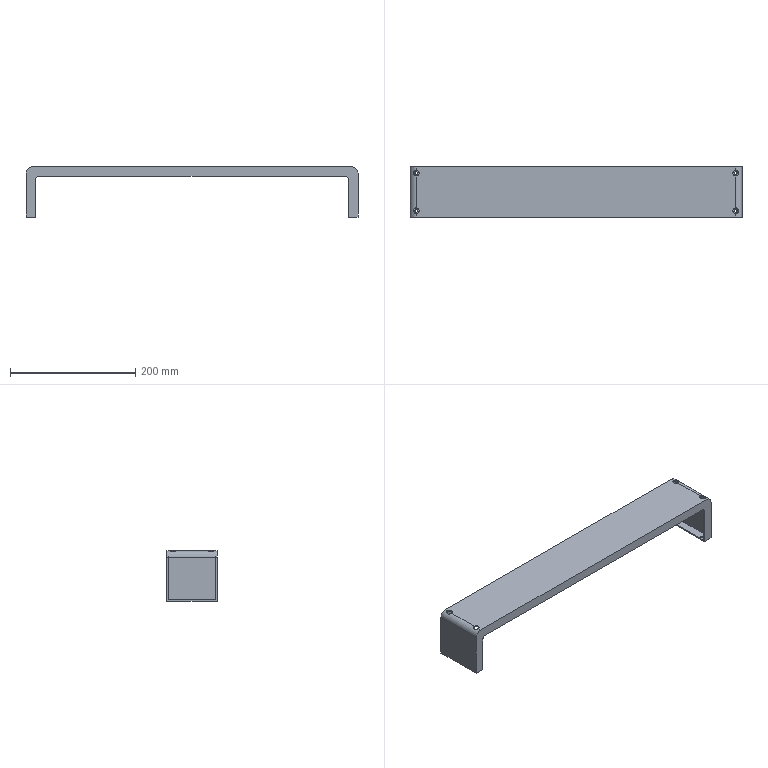Part | NX | 1 solid | 37 faces | box 530 x 80 x 80 mm | volume 145819 mm3 | cylinder 19 | plane 18 | commonest cylinder face diameters 4.5 x4 9 x4 10 x4 3.3 x3 16 x2 20 x2
STEP:
#1=CARTESIAN_POINT('',(-252.75,30.,-40.));
#2=VERTEX_POINT('',#1);
#3=CARTESIAN_POINT('',(-255.,30.,-40.));
#4=DIRECTION('',(0.,0.,1.));
#5=DIRECTION('',(1.,0.,0.));
#6=AXIS2_PLACEMENT_3D('',#3,#4,#5);
#7=CIRCLE('',#6,2.25);
#8=EDGE_CURVE('',#2,#2,#7,.T.);
#9=ORIENTED_EDGE('',*,*,#8,.T.);
#10=EDGE_LOOP('',(#9));
#11=FACE_BOUND('',#10,.T.);
#12=CARTESIAN_POINT('',(-252.75,-30.,-40.));
#13=VERTEX_POINT('',#12);
#14=CARTESIAN_POINT('',(-255.,-30.,-40.));
#15=DIRECTION('',(0.,0.,1.));
#16=DIRECTION('',(1.,0.,0.));
#17=AXIS2_PLACEMENT_3D('',#14,#15,#16);
#18=CIRCLE('',#17,2.25);
#19=EDGE_CURVE('',#13,#13,#18,.T.);
#20=ORIENTED_EDGE('',*,*,#19,.T.);
#21=EDGE_LOOP('',(#20));
#22=FACE_BOUND('',#21,.T.);
#23=CARTESIAN_POINT('',(-250.,40.,-40.));
#24=VERTEX_POINT('',#23);
#25=CARTESIAN_POINT('',(-265.,40.,-40.));
#26=VERTEX_POINT('',#25);
#27=CARTESIAN_POINT('',(-265.,40.,-40.));
#28=DIRECTION('',(-1.,0.,0.));
#29=VECTOR('',#28,1000.);
#30=LINE('',#27,#29);
#31=EDGE_CURVE('',#24,#26,#30,.T.);
#32=ORIENTED_EDGE('',*,*,#31,.F.);
#33=CARTESIAN_POINT('',(-250.,-40.,-40.));
#34=VERTEX_POINT('',#33);
#35=CARTESIAN_POINT('',(-250.,-40.,-40.));
#36=DIRECTION('',(0.,-1.,0.));
#37=VECTOR('',#36,1000.);
#38=LINE('',#35,#37);
#39=EDGE_CURVE('',#24,#34,#38,.T.);
#40=ORIENTED_EDGE('',*,*,#39,.T.);
#41=CARTESIAN_POINT('',(-265.,-40.,-40.));
#42=VERTEX_POINT('',#41);
#43=CARTESIAN_POINT('',(-265.,-40.,-40.));
#44=DIRECTION('',(-1.,0.,0.));
#45=VECTOR('',#44,1000.);
#46=LINE('',#43,#45);
#47=EDGE_CURVE('',#34,#42,#46,.T.);
#48=ORIENTED_EDGE('',*,*,#47,.T.);
#49=CARTESIAN_POINT('',(-265.,40.,-40.));
#50=DIRECTION('',(0.,-1.,0.));
#51=VECTOR('',#50,1000.);
#52=LINE('',#49,#51);
#53=EDGE_CURVE('',#26,#42,#52,.T.);
#54=ORIENTED_EDGE('',*,*,#53,.F.);
#55=EDGE_LOOP('',(#32,#40,#48,#54));
#56=FACE_BOUND('',#55,.T.);
#57=CARTESIAN_POINT('',(-265.,40.,-40.));
#58=DIRECTION('',(0.,0.,1.));
#59=DIRECTION('',(1.,0.,0.));
#60=AXIS2_PLACEMENT_3D('',#57,#58,#59);
#61=PLANE('',#60);
#62=ADVANCED_FACE('',(#11,#22,#56),#61,.F.);
#63=CARTESIAN_POINT('',(257.25,-30.,-40.));
#64=VERTEX_POINT('',#63);
#65=CARTESIAN_POINT('',(255.,-30.,-40.));
#66=DIRECTION('',(0.,0.,1.));
#67=DIRECTION('',(1.,0.,0.));
#68=AXIS2_PLACEMENT_3D('',#65,#66,#67);
#69=CIRCLE('',#68,2.25);
#70=EDGE_CURVE('',#64,#64,#69,.T.);
#71=ORIENTED_EDGE('',*,*,#70,.T.);
#72=EDGE_LOOP('',(#71));
#73=FACE_BOUND('',#72,.T.);
#74=CARTESIAN_POINT('',(257.25,30.,-40.));
#75=VERTEX_POINT('',#74);
#76=CARTESIAN_POINT('',(255.,30.,-40.));
#77=DIRECTION('',(0.,0.,1.));
#78=DIRECTION('',(1.,0.,0.));
#79=AXIS2_PLACEMENT_3D('',#76,#77,#78);
#80=CIRCLE('',#79,2.25);
#81=EDGE_CURVE('',#75,#75,#80,.T.);
#82=ORIENTED_EDGE('',*,*,#81,.T.);
#83=EDGE_LOOP('',(#82));
#84=FACE_BOUND('',#83,.T.);
#85=CARTESIAN_POINT('',(265.,-40.,-40.));
#86=VERTEX_POINT('',#85);
#87=CARTESIAN_POINT('',(250.,-40.,-40.));
#88=VERTEX_POINT('',#87);
#89=CARTESIAN_POINT('',(-265.,-40.,-40.));
#90=DIRECTION('',(-1.,0.,0.));
#91=VECTOR('',#90,1000.);
#92=LINE('',#89,#91);
#93=EDGE_CURVE('',#86,#88,#92,.T.);
#94=ORIENTED_EDGE('',*,*,#93,.T.);
#95=CARTESIAN_POINT('',(250.,40.,-40.));
#96=VERTEX_POINT('',#95);
#97=CARTESIAN_POINT('',(250.,-40.,-40.));
#98=DIRECTION('',(0.,1.,0.));
#99=VECTOR('',#98,1000.);
#100=LINE('',#97,#99);
#101=EDGE_CURVE('',#88,#96,#100,.T.);
#102=ORIENTED_EDGE('',*,*,#101,.T.);
#103=CARTESIAN_POINT('',(265.,40.,-40.));
#104=VERTEX_POINT('',#103);
#105=CARTESIAN_POINT('',(-265.,40.,-40.));
#106=DIRECTION('',(-1.,0.,0.));
#107=VECTOR('',#106,1000.);
#108=LINE('',#105,#107);
#109=EDGE_CURVE('',#104,#96,#108,.T.);
#110=ORIENTED_EDGE('',*,*,#109,.F.);
#111=CARTESIAN_POINT('',(265.,40.,-40.));
#112=DIRECTION('',(0.,-1.,0.));
#113=VECTOR('',#112,1000.);
#114=LINE('',#111,#113);
#115=EDGE_CURVE('',#104,#86,#114,.T.);
#116=ORIENTED_EDGE('',*,*,#115,.T.);
#117=EDGE_LOOP('',(#94,#102,#110,#116));
#118=FACE_BOUND('',#117,.T.);
#119=CARTESIAN_POINT('',(-265.,40.,-40.));
#120=DIRECTION('',(0.,0.,1.));
#121=DIRECTION('',(1.,0.,0.));
#122=AXIS2_PLACEMENT_3D('',#119,#120,#121);
#123=PLANE('',#122);
#124=ADVANCED_FACE('',(#73,#84,#118),#123,.F.);
#125=CARTESIAN_POINT('',(265.,-40.,30.));
#126=VERTEX_POINT('',#125);
#127=CARTESIAN_POINT('',(265.,-40.,-40.));
#128=DIRECTION('',(0.,0.,-1.));
#129=VECTOR('',#128,1000.);
#130=LINE('',#127,#129);
#131=EDGE_CURVE('',#126,#86,#130,.T.);
#132=ORIENTED_EDGE('',*,*,#131,.T.);
#133=ORIENTED_EDGE('',*,*,#115,.F.);
#134=CARTESIAN_POINT('',(265.,40.,30.));
#135=VERTEX_POINT('',#134);
#136=CARTESIAN_POINT('',(265.,40.,-40.));
#137=DIRECTION('',(0.,0.,-1.));
#138=VECTOR('',#137,1000.);
#139=LINE('',#136,#138);
#140=EDGE_CURVE('',#135,#104,#139,.T.);
#141=ORIENTED_EDGE('',*,*,#140,.F.);
#142=CARTESIAN_POINT('',(265.,40.,30.));
#143=DIRECTION('',(0.,-1.,0.));
#144=VECTOR('',#143,1000.);
#145=LINE('',#142,#144);
#146=EDGE_CURVE('',#135,#126,#145,.T.);
#147=ORIENTED_EDGE('',*,*,#146,.T.);
#148=EDGE_LOOP('',(#132,#133,#141,#147));
#149=FACE_BOUND('',#148,.T.);
#150=CARTESIAN_POINT('',(265.,40.,-40.));
#151=DIRECTION('',(-1.,0.,0.));
#152=DIRECTION('',(0.,0.,1.));
#153=AXIS2_PLACEMENT_3D('',#150,#151,#152);
#154=PLANE('',#153);
#155=ADVANCED_FACE('',(#149),#154,.F.);
#156=CARTESIAN_POINT('',(-265.,-40.,30.));
#157=VERTEX_POINT('',#156);
#158=CARTESIAN_POINT('',(-265.,40.,30.));
#159=VERTEX_POINT('',#158);
#160=CARTESIAN_POINT('',(-265.,40.,30.));
#161=DIRECTION('',(0.,-1.,0.));
#162=VECTOR('',#161,1000.);
#163=LINE('',#160,#162);
#164=EDGE_CURVE('',#157,#159,#163,.F.);
#165=ORIENTED_EDGE('',*,*,#164,.T.);
#166=CARTESIAN_POINT('',(-265.,40.,-40.));
#167=DIRECTION('',(0.,0.,1.));
#168=VECTOR('',#167,1000.);
#169=LINE('',#166,#168);
#170=EDGE_CURVE('',#26,#159,#169,.T.);
#171=ORIENTED_EDGE('',*,*,#170,.F.);
#172=ORIENTED_EDGE('',*,*,#53,.T.);
#173=CARTESIAN_POINT('',(-265.,-40.,-40.));
#174=DIRECTION('',(0.,0.,1.));
#175=VECTOR('',#174,1000.);
#176=LINE('',#173,#175);
#177=EDGE_CURVE('',#42,#157,#176,.T.);
#178=ORIENTED_EDGE('',*,*,#177,.T.);
#179=EDGE_LOOP('',(#165,#171,#172,#178));
#180=FACE_BOUND('',#179,.T.);
#181=CARTESIAN_POINT('',(-265.,40.,-40.));
#182=DIRECTION('',(1.,0.,0.));
#183=DIRECTION('',(0.,0.,-1.));
#184=AXIS2_PLACEMENT_3D('',#181,#182,#183);
#185=PLANE('',#184);
#186=ADVANCED_FACE('',(#180),#185,.F.);
#187=CARTESIAN_POINT('',(-255.,40.,40.));
#188=VERTEX_POINT('',#187);
#189=CARTESIAN_POINT('',(-255.,34.5,40.));
#190=VERTEX_POINT('',#189);
#191=CARTESIAN_POINT('',(-255.,40.,40.));
#192=DIRECTION('',(0.,-1.,0.));
#193=VECTOR('',#192,1000.);
#194=LINE('',#191,#193);
#195=EDGE_CURVE('',#188,#190,#194,.T.);
#196=ORIENTED_EDGE('',*,*,#195,.T.);
#197=CARTESIAN_POINT('',(-255.,25.5,40.));
#198=VERTEX_POINT('',#197);
#199=CARTESIAN_POINT('',(-255.,30.,40.));
#200=DIRECTION('',(0.,0.,1.));
#201=DIRECTION('',(1.,0.,0.));
#202=AXIS2_PLACEMENT_3D('',#199,#200,#201);
#203=CIRCLE('',#202,4.5);
#204=EDGE_CURVE('',#198,#190,#203,.T.);
#205=ORIENTED_EDGE('',*,*,#204,.F.);
#206=CARTESIAN_POINT('',(-255.,-25.5,40.));
#207=VERTEX_POINT('',#206);
#208=CARTESIAN_POINT('',(-255.,40.,40.));
#209=DIRECTION('',(0.,-1.,0.));
#210=VECTOR('',#209,1000.);
#211=LINE('',#208,#210);
#212=EDGE_CURVE('',#198,#207,#211,.T.);
#213=ORIENTED_EDGE('',*,*,#212,.T.);
#214=CARTESIAN_POINT('',(-255.,-34.5,40.));
#215=VERTEX_POINT('',#214);
#216=CARTESIAN_POINT('',(-255.,-30.,40.));
#217=DIRECTION('',(0.,0.,1.));
#218=DIRECTION('',(1.,0.,0.));
#219=AXIS2_PLACEMENT_3D('',#216,#217,#218);
#220=CIRCLE('',#219,4.5);
#221=EDGE_CURVE('',#215,#207,#220,.T.);
#222=ORIENTED_EDGE('',*,*,#221,.F.);
#223=CARTESIAN_POINT('',(-255.,-40.,40.));
#224=VERTEX_POINT('',#223);
#225=CARTESIAN_POINT('',(-255.,40.,40.));
#226=DIRECTION('',(0.,-1.,0.));
#227=VECTOR('',#226,1000.);
#228=LINE('',#225,#227);
#229=EDGE_CURVE('',#215,#224,#228,.T.);
#230=ORIENTED_EDGE('',*,*,#229,.T.);
#231=CARTESIAN_POINT('',(255.,-40.,40.));
#232=VERTEX_POINT('',#231);
#233=CARTESIAN_POINT('',(-265.,-40.,40.));
#234=DIRECTION('',(1.,0.,0.));
#235=VECTOR('',#234,1000.);
#236=LINE('',#233,#235);
#237=EDGE_CURVE('',#224,#232,#236,.T.);
#238=ORIENTED_EDGE('',*,*,#237,.T.);
#239=CARTESIAN_POINT('',(255.,-34.5,40.));
#240=VERTEX_POINT('',#239);
#241=CARTESIAN_POINT('',(255.,40.,40.));
#242=DIRECTION('',(0.,-1.,0.));
#243=VECTOR('',#242,1000.);
#244=LINE('',#241,#243);
#245=EDGE_CURVE('',#232,#240,#244,.F.);
#246=ORIENTED_EDGE('',*,*,#245,.T.);
#247=CARTESIAN_POINT('',(255.,-25.5,40.));
#248=VERTEX_POINT('',#247);
#249=CARTESIAN_POINT('',(255.,-30.,40.));
#250=DIRECTION('',(0.,0.,1.));
#251=DIRECTION('',(1.,0.,0.));
#252=AXIS2_PLACEMENT_3D('',#249,#250,#251);
#253=CIRCLE('',#252,4.5);
#254=EDGE_CURVE('',#248,#240,#253,.T.);
#255=ORIENTED_EDGE('',*,*,#254,.F.);
#256=CARTESIAN_POINT('',(255.,25.5,40.));
#257=VERTEX_POINT('',#256);
#258=CARTESIAN_POINT('',(255.,40.,40.));
#259=DIRECTION('',(0.,-1.,0.));
#260=VECTOR('',#259,1000.);
#261=LINE('',#258,#260);
#262=EDGE_CURVE('',#248,#257,#261,.F.);
#263=ORIENTED_EDGE('',*,*,#262,.T.);
#264=CARTESIAN_POINT('',(255.,34.5,40.));
#265=VERTEX_POINT('',#264);
#266=CARTESIAN_POINT('',(255.,30.,40.));
#267=DIRECTION('',(0.,0.,1.));
#268=DIRECTION('',(1.,0.,0.));
#269=AXIS2_PLACEMENT_3D('',#266,#267,#268);
#270=CIRCLE('',#269,4.5);
#271=EDGE_CURVE('',#265,#257,#270,.T.);
#272=ORIENTED_EDGE('',*,*,#271,.F.);
#273=CARTESIAN_POINT('',(255.,40.,40.));
#274=VERTEX_POINT('',#273);
#275=CARTESIAN_POINT('',(255.,40.,40.));
#276=DIRECTION('',(0.,-1.,0.));
#277=VECTOR('',#276,1000.);
#278=LINE('',#275,#277);
#279=EDGE_CURVE('',#265,#274,#278,.F.);
#280=ORIENTED_EDGE('',*,*,#279,.T.);
#281=CARTESIAN_POINT('',(-265.,40.,40.));
#282=DIRECTION('',(1.,0.,0.));
#283=VECTOR('',#282,1000.);
#284=LINE('',#281,#283);
#285=EDGE_CURVE('',#188,#274,#284,.T.);
#286=ORIENTED_EDGE('',*,*,#285,.F.);
#287=EDGE_LOOP('',(#196,#205,#213,#222,#230,#238,#246,#255,#263,#272,#280,#286));
#288=FACE_BOUND('',#287,.T.);
#289=CARTESIAN_POINT('',(-265.,40.,40.));
#290=DIRECTION('',(0.,0.,-1.));
#291=DIRECTION('',(-1.,0.,0.));
#292=AXIS2_PLACEMENT_3D('',#289,#290,#291);
#293=PLANE('',#292);
#294=ADVANCED_FACE('',(#288),#293,.F.);
#295=CARTESIAN_POINT('',(-255.,40.,31.65));
#296=VERTEX_POINT('',#295);
#297=CARTESIAN_POINT('',(-255.,40.,30.));
#298=DIRECTION('',(0.,1.,0.));
#299=DIRECTION('',(0.,0.,1.));
#300=AXIS2_PLACEMENT_3D('',#297,#298,#299);
#301=CIRCLE('',#300,1.65);
#302=EDGE_CURVE('',#296,#296,#301,.T.);
#303=ORIENTED_EDGE('',*,*,#302,.F.);
#304=EDGE_LOOP('',(#303));
#305=FACE_BOUND('',#304,.T.);
#306=CARTESIAN_POINT('',(0.,40.,31.65));
#307=VERTEX_POINT('',#306);
#308=CARTESIAN_POINT('',(0.,40.,30.));
#309=DIRECTION('',(0.,1.,0.));
#310=DIRECTION('',(0.,0.,1.));
#311=AXIS2_PLACEMENT_3D('',#308,#309,#310);
#312=CIRCLE('',#311,1.65);
#313=EDGE_CURVE('',#307,#307,#312,.T.);
#314=ORIENTED_EDGE('',*,*,#313,.F.);
#315=EDGE_LOOP('',(#314));
#316=FACE_BOUND('',#315,.T.);
#317=CARTESIAN_POINT('',(255.,40.,31.65));
#318=VERTEX_POINT('',#317);
#319=CARTESIAN_POINT('',(255.,40.,30.));
#320=DIRECTION('',(0.,1.,0.));
#321=DIRECTION('',(0.,0.,1.));
#322=AXIS2_PLACEMENT_3D('',#319,#320,#321);
#323=CIRCLE('',#322,1.65);
#324=EDGE_CURVE('',#318,#318,#323,.T.);
#325=ORIENTED_EDGE('',*,*,#324,.F.);
#326=EDGE_LOOP('',(#325));
#327=FACE_BOUND('',#326,.T.);
#328=CARTESIAN_POINT('',(-250.,40.,20.));
#329=VERTEX_POINT('',#328);
#330=CARTESIAN_POINT('',(-250.,40.,-40.));
#331=DIRECTION('',(0.,0.,1.));
#332=VECTOR('',#331,1000.);
#333=LINE('',#330,#332);
#334=EDGE_CURVE('',#24,#329,#333,.T.);
#335=ORIENTED_EDGE('',*,*,#334,.F.);
#336=ORIENTED_EDGE('',*,*,#31,.T.);
#337=ORIENTED_EDGE('',*,*,#170,.T.);
#338=CARTESIAN_POINT('',(-255.,40.,30.));
#339=DIRECTION('',(0.,1.,0.));
#340=DIRECTION('',(0.,0.,1.));
#341=AXIS2_PLACEMENT_3D('',#338,#339,#340);
#342=CIRCLE('',#341,10.);
#343=EDGE_CURVE('',#159,#188,#342,.T.);
#344=ORIENTED_EDGE('',*,*,#343,.T.);
#345=ORIENTED_EDGE('',*,*,#285,.T.);
#346=CARTESIAN_POINT('',(255.,40.,30.));
#347=DIRECTION('',(0.,1.,0.));
#348=DIRECTION('',(0.,0.,1.));
#349=AXIS2_PLACEMENT_3D('',#346,#347,#348);
#350=CIRCLE('',#349,10.);
#351=EDGE_CURVE('',#274,#135,#350,.T.);
#352=ORIENTED_EDGE('',*,*,#351,.T.);
#353=ORIENTED_EDGE('',*,*,#140,.T.);
#354=ORIENTED_EDGE('',*,*,#109,.T.);
#355=CARTESIAN_POINT('',(250.,40.,20.));
#356=VERTEX_POINT('',#355);
#357=CARTESIAN_POINT('',(250.,40.,-40.));
#358=DIRECTION('',(0.,0.,-1.));
#359=VECTOR('',#358,1000.);
#360=LINE('',#357,#359);
#361=EDGE_CURVE('',#356,#96,#360,.T.);
#362=ORIENTED_EDGE('',*,*,#361,.F.);
#363=CARTESIAN_POINT('',(245.,40.,25.));
#364=VERTEX_POINT('',#363);
#365=CARTESIAN_POINT('',(245.,40.,20.));
#366=DIRECTION('',(0.,1.,0.));
#367=DIRECTION('',(0.,0.,-1.));
#368=AXIS2_PLACEMENT_3D('',#365,#366,#367);
#369=CIRCLE('',#368,5.);
#370=EDGE_CURVE('',#364,#356,#369,.T.);
#371=ORIENTED_EDGE('',*,*,#370,.F.);
#372=CARTESIAN_POINT('',(-245.,40.,25.));
#373=VERTEX_POINT('',#372);
#374=CARTESIAN_POINT('',(-245.,40.,25.));
#375=DIRECTION('',(1.,0.,0.));
#376=VECTOR('',#375,1000.);
#377=LINE('',#374,#376);
#378=EDGE_CURVE('',#373,#364,#377,.T.);
#379=ORIENTED_EDGE('',*,*,#378,.F.);
#380=CARTESIAN_POINT('',(-245.,40.,20.));
#381=DIRECTION('',(0.,1.,0.));
#382=DIRECTION('',(0.,0.,-1.));
#383=AXIS2_PLACEMENT_3D('',#380,#381,#382);
#384=CIRCLE('',#383,5.);
#385=EDGE_CURVE('',#329,#373,#384,.T.);
#386=ORIENTED_EDGE('',*,*,#385,.F.);
#387=EDGE_LOOP('',(#335,#336,#337,#344,#345,#352,#353,#354,#362,#371,#379,#386));
#388=FACE_BOUND('',#387,.T.);
#389=CARTESIAN_POINT('',(0.,40.,0.));
#390=DIRECTION('',(0.,1.,0.));
#391=DIRECTION('',(0.,0.,1.));
#392=AXIS2_PLACEMENT_3D('',#389,#390,#391);
#393=PLANE('',#392);
#394=ADVANCED_FACE('',(#305,#316,#327,#388),#393,.T.);
#395=ORIENTED_EDGE('',*,*,#47,.F.);
#396=CARTESIAN_POINT('',(-250.,-40.,20.));
#397=VERTEX_POINT('',#396);
#398=CARTESIAN_POINT('',(-250.,-40.,-40.));
#399=DIRECTION('',(0.,0.,1.));
#400=VECTOR('',#399,1000.);
#401=LINE('',#398,#400);
#402=EDGE_CURVE('',#34,#397,#401,.T.);
#403=ORIENTED_EDGE('',*,*,#402,.T.);
#404=CARTESIAN_POINT('',(-245.,-40.,25.));
#405=VERTEX_POINT('',#404);
#406=CARTESIAN_POINT('',(-245.,-40.,20.));
#407=DIRECTION('',(0.,1.,0.));
#408=DIRECTION('',(0.,0.,-1.));
#409=AXIS2_PLACEMENT_3D('',#406,#407,#408);
#410=CIRCLE('',#409,5.);
#411=EDGE_CURVE('',#397,#405,#410,.T.);
#412=ORIENTED_EDGE('',*,*,#411,.T.);
#413=CARTESIAN_POINT('',(245.,-40.,25.));
#414=VERTEX_POINT('',#413);
#415=CARTESIAN_POINT('',(-245.,-40.,25.));
#416=DIRECTION('',(1.,0.,0.));
#417=VECTOR('',#416,1000.);
#418=LINE('',#415,#417);
#419=EDGE_CURVE('',#405,#414,#418,.T.);
#420=ORIENTED_EDGE('',*,*,#419,.T.);
#421=CARTESIAN_POINT('',(250.,-40.,20.));
#422=VERTEX_POINT('',#421);
#423=CARTESIAN_POINT('',(245.,-40.,20.));
#424=DIRECTION('',(0.,1.,0.));
#425=DIRECTION('',(0.,0.,-1.));
#426=AXIS2_PLACEMENT_3D('',#423,#424,#425);
#427=CIRCLE('',#426,5.);
#428=EDGE_CURVE('',#414,#422,#427,.T.);
#429=ORIENTED_EDGE('',*,*,#428,.T.);
#430=CARTESIAN_POINT('',(250.,-40.,-40.));
#431=DIRECTION('',(0.,0.,-1.));
#432=VECTOR('',#431,1000.);
#433=LINE('',#430,#432);
#434=EDGE_CURVE('',#422,#88,#433,.T.);
#435=ORIENTED_EDGE('',*,*,#434,.T.);
#436=ORIENTED_EDGE('',*,*,#93,.F.);
#437=ORIENTED_EDGE('',*,*,#131,.F.);
#438=CARTESIAN_POINT('',(255.,-40.,30.));
#439=DIRECTION('',(0.,1.,0.));
#440=DIRECTION('',(0.,0.,1.));
#441=AXIS2_PLACEMENT_3D('',#438,#439,#440);
#442=CIRCLE('',#441,10.);
#443=EDGE_CURVE('',#126,#232,#442,.F.);
#444=ORIENTED_EDGE('',*,*,#443,.T.);
#445=ORIENTED_EDGE('',*,*,#237,.F.);
#446=CARTESIAN_POINT('',(-255.,-40.,30.));
#447=DIRECTION('',(0.,1.,0.));
#448=DIRECTION('',(0.,0.,1.));
#449=AXIS2_PLACEMENT_3D('',#446,#447,#448);
#450=CIRCLE('',#449,10.);
#451=EDGE_CURVE('',#224,#157,#450,.F.);
#452=ORIENTED_EDGE('',*,*,#451,.T.);
#453=ORIENTED_EDGE('',*,*,#177,.F.);
#454=EDGE_LOOP('',(#395,#403,#412,#420,#429,#435,#436,#437,#444,#445,#452,#453));
#455=FACE_BOUND('',#454,.T.);
#456=CARTESIAN_POINT('',(0.,-40.,0.));
#457=DIRECTION('',(0.,1.,0.));
#458=DIRECTION('',(0.,0.,1.));
#459=AXIS2_PLACEMENT_3D('',#456,#457,#458);
#460=PLANE('',#459);
#461=ADVANCED_FACE('',(#455),#460,.F.);
#462=CARTESIAN_POINT('',(-255.,34.5,40.));
#463=CARTESIAN_POINT('',(-256.206,34.5,40.));
#464=CARTESIAN_POINT('',(-258.514,33.52,39.494));
#465=CARTESIAN_POINT('',(-259.992,30.011,38.648));
#466=CARTESIAN_POINT('',(-258.516,26.475,39.493));
#467=CARTESIAN_POINT('',(-256.207,25.5,40.));
#468=CARTESIAN_POINT('',(-255.,25.5,40.));
#469=B_SPLINE_CURVE_WITH_KNOTS('',3,(#462,#463,#464,#465,#466,#467,#468),.UNSPECIFIED.,.F.,.F.,(4,1,1,1,4),(0.,0.003564,0.007128,0.01069,0.01426),.UNSPECIFIED.);
#470=EDGE_CURVE('',#190,#198,#469,.T.);
#471=ORIENTED_EDGE('',*,*,#470,.F.);
#472=ORIENTED_EDGE('',*,*,#195,.F.);
#473=ORIENTED_EDGE('',*,*,#343,.F.);
#474=ORIENTED_EDGE('',*,*,#164,.F.);
#475=ORIENTED_EDGE('',*,*,#451,.F.);
#476=ORIENTED_EDGE('',*,*,#229,.F.);
#477=CARTESIAN_POINT('',(-255.,-25.5,40.));
#478=CARTESIAN_POINT('',(-256.206,-25.5,40.));
#479=CARTESIAN_POINT('',(-258.514,-26.48,39.494));
#480=CARTESIAN_POINT('',(-259.992,-29.989,38.648));
#481=CARTESIAN_POINT('',(-258.516,-33.525,39.493));
#482=CARTESIAN_POINT('',(-256.207,-34.5,40.));
#483=CARTESIAN_POINT('',(-255.,-34.5,40.));
#484=B_SPLINE_CURVE_WITH_KNOTS('',3,(#477,#478,#479,#480,#481,#482,#483),.UNSPECIFIED.,.F.,.F.,(4,1,1,1,4),(0.,0.003564,0.007128,0.01069,0.01426),.UNSPECIFIED.);
#485=EDGE_CURVE('',#207,#215,#484,.T.);
#486=ORIENTED_EDGE('',*,*,#485,.F.);
#487=ORIENTED_EDGE('',*,*,#212,.F.);
#488=EDGE_LOOP('',(#471,#472,#473,#474,#475,#476,#486,#487));
#489=FACE_BOUND('',#488,.T.);
#490=CARTESIAN_POINT('',(-255.,40.,30.));
#491=DIRECTION('',(0.,-1.,0.));
#492=DIRECTION('',(0.,0.,-1.));
#493=AXIS2_PLACEMENT_3D('',#490,#491,#492);
#494=CYLINDRICAL_SURFACE('',#493,10.);
#495=ADVANCED_FACE('',(#489),#494,.T.);
#496=CARTESIAN_POINT('',(255.,-34.5,40.));
#497=CARTESIAN_POINT('',(256.206,-34.5,40.));
#498=CARTESIAN_POINT('',(258.514,-33.52,39.494));
#499=CARTESIAN_POINT('',(259.992,-30.011,38.648));
#500=CARTESIAN_POINT('',(258.516,-26.475,39.493));
#501=CARTESIAN_POINT('',(256.207,-25.5,40.));
#502=CARTESIAN_POINT('',(255.,-25.5,40.));
#503=B_SPLINE_CURVE_WITH_KNOTS('',3,(#496,#497,#498,#499,#500,#501,#502),.UNSPECIFIED.,.F.,.F.,(4,1,1,1,4),(0.,0.003564,0.007128,0.01069,0.01426),.UNSPECIFIED.);
#504=EDGE_CURVE('',#240,#248,#503,.T.);
#505=ORIENTED_EDGE('',*,*,#504,.F.);
#506=ORIENTED_EDGE('',*,*,#245,.F.);
#507=ORIENTED_EDGE('',*,*,#443,.F.);
#508=ORIENTED_EDGE('',*,*,#146,.F.);
#509=ORIENTED_EDGE('',*,*,#351,.F.);
#510=ORIENTED_EDGE('',*,*,#279,.F.);
#511=CARTESIAN_POINT('',(255.,25.5,40.));
#512=CARTESIAN_POINT('',(256.206,25.5,40.));
#513=CARTESIAN_POINT('',(258.514,26.48,39.494));
#514=CARTESIAN_POINT('',(259.992,29.989,38.648));
#515=CARTESIAN_POINT('',(258.516,33.525,39.493));
#516=CARTESIAN_POINT('',(256.207,34.5,40.));
#517=CARTESIAN_POINT('',(255.,34.5,40.));
#518=B_SPLINE_CURVE_WITH_KNOTS('',3,(#511,#512,#513,#514,#515,#516,#517),.UNSPECIFIED.,.F.,.F.,(4,1,1,1,4),(0.,0.003564,0.007128,0.01069,0.01426),.UNSPECIFIED.);
#519=EDGE_CURVE('',#257,#265,#518,.T.);
#520=ORIENTED_EDGE('',*,*,#519,.F.);
#521=ORIENTED_EDGE('',*,*,#262,.F.);
#522=EDGE_LOOP('',(#505,#506,#507,#508,#509,#510,#520,#521));
#523=FACE_BOUND('',#522,.T.);
#524=CARTESIAN_POINT('',(255.,40.,30.));
#525=DIRECTION('',(0.,-1.,0.));
#526=DIRECTION('',(0.,0.,-1.));
#527=AXIS2_PLACEMENT_3D('',#524,#525,#526);
#528=CYLINDRICAL_SURFACE('',#527,10.);
#529=ADVANCED_FACE('',(#523),#528,.T.);
#530=CARTESIAN_POINT('',(263.,-38.,-38.));
#531=VERTEX_POINT('',#530);
#532=CARTESIAN_POINT('',(263.,38.,-38.));
#533=VERTEX_POINT('',#532);
#534=CARTESIAN_POINT('',(263.,40.,-38.));
#535=DIRECTION('',(0.,1.,0.));
#536=VECTOR('',#535,1000.);
#537=LINE('',#534,#536);
#538=EDGE_CURVE('',#531,#533,#537,.T.);
#539=ORIENTED_EDGE('',*,*,#538,.F.);
#540=CARTESIAN_POINT('',(263.,-38.,30.));
#541=VERTEX_POINT('',#540);
#542=CARTESIAN_POINT('',(263.,-38.,-40.));
#543=DIRECTION('',(0.,0.,-1.));
#544=VECTOR('',#543,1000.);
#545=LINE('',#542,#544);
#546=EDGE_CURVE('',#541,#531,#545,.T.);
#547=ORIENTED_EDGE('',*,*,#546,.F.);
#548=CARTESIAN_POINT('',(263.,38.,30.));
#549=VERTEX_POINT('',#548);
#550=CARTESIAN_POINT('',(263.,40.,30.));
#551=DIRECTION('',(0.,1.,0.));
#552=VECTOR('',#551,1000.);
#553=LINE('',#550,#552);
#554=EDGE_CURVE('',#549,#541,#553,.F.);
#555=ORIENTED_EDGE('',*,*,#554,.F.);
#556=CARTESIAN_POINT('',(263.,38.,-40.));
#557=DIRECTION('',(0.,0.,-1.));
#558=VECTOR('',#557,1000.);
#559=LINE('',#556,#558);
#560=EDGE_CURVE('',#549,#533,#559,.T.);
#561=ORIENTED_EDGE('',*,*,#560,.T.);
#562=EDGE_LOOP('',(#539,#547,#555,#561));
#563=FACE_BOUND('',#562,.T.);
#564=CARTESIAN_POINT('',(263.,40.,-40.));
#565=DIRECTION('',(-1.,0.,0.));
#566=DIRECTION('',(0.,0.,1.));
#567=AXIS2_PLACEMENT_3D('',#564,#565,#566);
#568=PLANE('',#567);
#569=ADVANCED_FACE('',(#563),#568,.T.);
#570=CARTESIAN_POINT('',(-263.,38.,-38.));
#571=VERTEX_POINT('',#570);
#572=CARTESIAN_POINT('',(-263.,-38.,-38.));
#573=VERTEX_POINT('',#572);
#574=CARTESIAN_POINT('',(-263.,40.,-38.));
#575=DIRECTION('',(0.,-1.,0.));
#576=VECTOR('',#575,1000.);
#577=LINE('',#574,#576);
#578=EDGE_CURVE('',#571,#573,#577,.T.);
#579=ORIENTED_EDGE('',*,*,#578,.F.);
#580=CARTESIAN_POINT('',(-263.,38.,30.));
#581=VERTEX_POINT('',#580);
#582=CARTESIAN_POINT('',(-263.,38.,-40.));
#583=DIRECTION('',(0.,0.,1.));
#584=VECTOR('',#583,1000.);
#585=LINE('',#582,#584);
#586=EDGE_CURVE('',#571,#581,#585,.T.);
#587=ORIENTED_EDGE('',*,*,#586,.T.);
#588=CARTESIAN_POINT('',(-263.,-38.,30.));
#589=VERTEX_POINT('',#588);
#590=CARTESIAN_POINT('',(-263.,40.,30.));
#591=DIRECTION('',(0.,1.,0.));
#592=VECTOR('',#591,1000.);
#593=LINE('',#590,#592);
#594=EDGE_CURVE('',#589,#581,#593,.T.);
#595=ORIENTED_EDGE('',*,*,#594,.F.);
#596=CARTESIAN_POINT('',(-263.,-38.,-40.));
#597=DIRECTION('',(0.,0.,1.));
#598=VECTOR('',#597,1000.);
#599=LINE('',#596,#598);
#600=EDGE_CURVE('',#573,#589,#599,.T.);
#601=ORIENTED_EDGE('',*,*,#600,.F.);
#602=EDGE_LOOP('',(#579,#587,#595,#601));
#603=FACE_BOUND('',#602,.T.);
#604=CARTESIAN_POINT('',(-263.,40.,-40.));
#605=DIRECTION('',(1.,0.,0.));
#606=DIRECTION('',(0.,0.,-1.));
#607=AXIS2_PLACEMENT_3D('',#604,#605,#606);
#608=PLANE('',#607);
#609=ADVANCED_FACE('',(#603),#608,.T.);
#610=CARTESIAN_POINT('',(-255.,34.5,38.));
#611=VERTEX_POINT('',#610);
#612=CARTESIAN_POINT('',(-255.,25.5,38.));
#613=VERTEX_POINT('',#612);
#614=CARTESIAN_POINT('',(-255.,30.,38.));
#615=DIRECTION('',(0.,0.,-1.));
#616=DIRECTION('',(-1.,0.,0.));
#617=AXIS2_PLACEMENT_3D('',#614,#615,#616);
#618=CIRCLE('',#617,4.5);
#619=EDGE_CURVE('',#611,#613,#618,.T.);
#620=ORIENTED_EDGE('',*,*,#619,.F.);
#621=CARTESIAN_POINT('',(-255.,38.,38.));
#622=VERTEX_POINT('',#621);
#623=CARTESIAN_POINT('',(-255.,40.,38.));
#624=DIRECTION('',(0.,1.,0.));
#625=VECTOR('',#624,1000.);
#626=LINE('',#623,#625);
#627=EDGE_CURVE('',#622,#611,#626,.F.);
#628=ORIENTED_EDGE('',*,*,#627,.F.);
#629=CARTESIAN_POINT('',(255.,38.,38.));
#630=VERTEX_POINT('',#629);
#631=CARTESIAN_POINT('',(-265.,38.,38.));
#632=DIRECTION('',(1.,0.,0.));
#633=VECTOR('',#632,1000.);
#634=LINE('',#631,#633);
#635=EDGE_CURVE('',#622,#630,#634,.T.);
#636=ORIENTED_EDGE('',*,*,#635,.T.);
#637=CARTESIAN_POINT('',(255.,34.5,38.));
#638=VERTEX_POINT('',#637);
#639=CARTESIAN_POINT('',(255.,40.,38.));
#640=DIRECTION('',(0.,1.,0.));
#641=VECTOR('',#640,1000.);
#642=LINE('',#639,#641);
#643=EDGE_CURVE('',#638,#630,#642,.T.);
#644=ORIENTED_EDGE('',*,*,#643,.F.);
#645=CARTESIAN_POINT('',(255.,25.5,38.));
#646=VERTEX_POINT('',#645);
#647=CARTESIAN_POINT('',(255.,30.,38.));
#648=DIRECTION('',(0.,0.,-1.));
#649=DIRECTION('',(-1.,0.,0.));
#650=AXIS2_PLACEMENT_3D('',#647,#648,#649);
#651=CIRCLE('',#650,4.5);
#652=EDGE_CURVE('',#646,#638,#651,.T.);
#653=ORIENTED_EDGE('',*,*,#652,.F.);
#654=CARTESIAN_POINT('',(255.,-25.5,38.));
#655=VERTEX_POINT('',#654);
#656=CARTESIAN_POINT('',(255.,40.,38.));
#657=DIRECTION('',(0.,1.,0.));
#658=VECTOR('',#657,1000.);
#659=LINE('',#656,#658);
#660=EDGE_CURVE('',#655,#646,#659,.T.);
#661=ORIENTED_EDGE('',*,*,#660,.F.);
#662=CARTESIAN_POINT('',(255.,-34.5,38.));
#663=VERTEX_POINT('',#662);
#664=CARTESIAN_POINT('',(255.,-30.,38.));
#665=DIRECTION('',(0.,0.,-1.));
#666=DIRECTION('',(-1.,0.,0.));
#667=AXIS2_PLACEMENT_3D('',#664,#665,#666);
#668=CIRCLE('',#667,4.5);
#669=EDGE_CURVE('',#663,#655,#668,.T.);
#670=ORIENTED_EDGE('',*,*,#669,.F.);
#671=CARTESIAN_POINT('',(255.,-38.,38.));
#672=VERTEX_POINT('',#671);
#673=CARTESIAN_POINT('',(255.,40.,38.));
#674=DIRECTION('',(0.,1.,0.));
#675=VECTOR('',#674,1000.);
#676=LINE('',#673,#675);
#677=EDGE_CURVE('',#672,#663,#676,.T.);
#678=ORIENTED_EDGE('',*,*,#677,.F.);
#679=CARTESIAN_POINT('',(-255.,-38.,38.));
#680=VERTEX_POINT('',#679);
#681=CARTESIAN_POINT('',(-265.,-38.,38.));
#682=DIRECTION('',(1.,0.,0.));
#683=VECTOR('',#682,1000.);
#684=LINE('',#681,#683);
#685=EDGE_CURVE('',#680,#672,#684,.T.);
#686=ORIENTED_EDGE('',*,*,#685,.F.);
#687=CARTESIAN_POINT('',(-255.,-34.5,38.));
#688=VERTEX_POINT('',#687);
#689=CARTESIAN_POINT('',(-255.,40.,38.));
#690=DIRECTION('',(0.,1.,0.));
#691=VECTOR('',#690,1000.);
#692=LINE('',#689,#691);
#693=EDGE_CURVE('',#688,#680,#692,.F.);
#694=ORIENTED_EDGE('',*,*,#693,.F.);
#695=CARTESIAN_POINT('',(-255.,-25.5,38.));
#696=VERTEX_POINT('',#695);
#697=CARTESIAN_POINT('',(-255.,-30.,38.));
#698=DIRECTION('',(0.,0.,-1.));
#699=DIRECTION('',(-1.,0.,0.));
#700=AXIS2_PLACEMENT_3D('',#697,#698,#699);
#701=CIRCLE('',#700,4.5);
#702=EDGE_CURVE('',#696,#688,#701,.T.);
#703=ORIENTED_EDGE('',*,*,#702,.F.);
#704=CARTESIAN_POINT('',(-255.,40.,38.));
#705=DIRECTION('',(0.,1.,0.));
#706=VECTOR('',#705,1000.);
#707=LINE('',#704,#706);
#708=EDGE_CURVE('',#613,#696,#707,.F.);
#709=ORIENTED_EDGE('',*,*,#708,.F.);
#710=EDGE_LOOP('',(#620,#628,#636,#644,#653,#661,#670,#678,#686,#694,#703,#709));
#711=FACE_BOUND('',#710,.T.);
#712=CARTESIAN_POINT('',(-265.,40.,38.));
#713=DIRECTION('',(0.,0.,-1.));
#714=DIRECTION('',(-1.,0.,0.));
#715=AXIS2_PLACEMENT_3D('',#712,#713,#714);
#716=PLANE('',#715);
#717=ADVANCED_FACE('',(#711),#716,.T.);
#718=CARTESIAN_POINT('',(-255.,38.,31.65));
#719=VERTEX_POINT('',#718);
#720=CARTESIAN_POINT('',(-255.,38.,30.));
#721=DIRECTION('',(0.,1.,0.));
#722=DIRECTION('',(0.,0.,1.));
#723=AXIS2_PLACEMENT_3D('',#720,#721,#722);
#724=CIRCLE('',#723,1.65);
#725=EDGE_CURVE('',#719,#719,#724,.T.);
#726=ORIENTED_EDGE('',*,*,#725,.T.);
#727=EDGE_LOOP('',(#726));
#728=FACE_BOUND('',#727,.T.);
#729=CARTESIAN_POINT('',(0.,38.,31.65));
#730=VERTEX_POINT('',#729);
#731=CARTESIAN_POINT('',(0.,38.,30.));
#732=DIRECTION('',(0.,1.,0.));
#733=DIRECTION('',(0.,0.,1.));
#734=AXIS2_PLACEMENT_3D('',#731,#732,#733);
#735=CIRCLE('',#734,1.65);
#736=EDGE_CURVE('',#730,#730,#735,.T.);
#737=ORIENTED_EDGE('',*,*,#736,.T.);
#738=EDGE_LOOP('',(#737));
#739=FACE_BOUND('',#738,.T.);
#740=CARTESIAN_POINT('',(255.,38.,31.65));
#741=VERTEX_POINT('',#740);
#742=CARTESIAN_POINT('',(255.,38.,30.));
#743=DIRECTION('',(0.,1.,0.));
#744=DIRECTION('',(0.,0.,1.));
#745=AXIS2_PLACEMENT_3D('',#742,#743,#744);
#746=CIRCLE('',#745,1.65);
#747=EDGE_CURVE('',#741,#741,#746,.T.);
#748=ORIENTED_EDGE('',*,*,#747,.T.);
#749=EDGE_LOOP('',(#748));
#750=FACE_BOUND('',#749,.T.);
#751=CARTESIAN_POINT('',(-250.,38.,-38.));
#752=VERTEX_POINT('',#751);
#753=CARTESIAN_POINT('',(0.,38.,-38.));
#754=DIRECTION('',(1.,0.,0.));
#755=VECTOR('',#754,1000.);
#756=LINE('',#753,#755);
#757=EDGE_CURVE('',#571,#752,#756,.T.);
#758=ORIENTED_EDGE('',*,*,#757,.T.);
#759=CARTESIAN_POINT('',(-250.,38.,20.));
#760=VERTEX_POINT('',#759);
#761=CARTESIAN_POINT('',(-250.,38.,0.));
#762=DIRECTION('',(0.,0.,1.));
#763=VECTOR('',#762,1000.);
#764=LINE('',#761,#763);
#765=EDGE_CURVE('',#752,#760,#764,.T.);
#766=ORIENTED_EDGE('',*,*,#765,.T.);
#767=CARTESIAN_POINT('',(-245.,38.,25.));
#768=VERTEX_POINT('',#767);
#769=CARTESIAN_POINT('',(-245.,38.,20.));
#770=DIRECTION('',(0.,1.,0.));
#771=DIRECTION('',(0.,0.,1.));
#772=AXIS2_PLACEMENT_3D('',#769,#770,#771);
#773=CIRCLE('',#772,5.);
#774=EDGE_CURVE('',#760,#768,#773,.T.);
#775=ORIENTED_EDGE('',*,*,#774,.T.);
#776=CARTESIAN_POINT('',(245.,38.,25.));
#777=VERTEX_POINT('',#776);
#778=CARTESIAN_POINT('',(0.,38.,25.));
#779=DIRECTION('',(1.,0.,0.));
#780=VECTOR('',#779,1000.);
#781=LINE('',#778,#780);
#782=EDGE_CURVE('',#768,#777,#781,.T.);
#783=ORIENTED_EDGE('',*,*,#782,.T.);
#784=CARTESIAN_POINT('',(250.,38.,20.));
#785=VERTEX_POINT('',#784);
#786=CARTESIAN_POINT('',(245.,38.,20.));
#787=DIRECTION('',(0.,1.,0.));
#788=DIRECTION('',(0.,0.,1.));
#789=AXIS2_PLACEMENT_3D('',#786,#787,#788);
#790=CIRCLE('',#789,5.);
#791=EDGE_CURVE('',#777,#785,#790,.T.);
#792=ORIENTED_EDGE('',*,*,#791,.T.);
#793=CARTESIAN_POINT('',(250.,38.,-38.));
#794=VERTEX_POINT('',#793);
#795=CARTESIAN_POINT('',(250.,38.,0.));
#796=DIRECTION('',(0.,0.,-1.));
#797=VECTOR('',#796,1000.);
#798=LINE('',#795,#797);
#799=EDGE_CURVE('',#785,#794,#798,.T.);
#800=ORIENTED_EDGE('',*,*,#799,.T.);
#801=CARTESIAN_POINT('',(0.,38.,-38.));
#802=DIRECTION('',(1.,0.,0.));
#803=VECTOR('',#802,1000.);
#804=LINE('',#801,#803);
#805=EDGE_CURVE('',#794,#533,#804,.T.);
#806=ORIENTED_EDGE('',*,*,#805,.T.);
#807=ORIENTED_EDGE('',*,*,#560,.F.);
#808=CARTESIAN_POINT('',(255.,38.,30.));
#809=DIRECTION('',(0.,1.,0.));
#810=DIRECTION('',(0.,0.,1.));
#811=AXIS2_PLACEMENT_3D('',#808,#809,#810);
#812=CIRCLE('',#811,8.);
#813=EDGE_CURVE('',#630,#549,#812,.T.);
#814=ORIENTED_EDGE('',*,*,#813,.F.);
#815=ORIENTED_EDGE('',*,*,#635,.F.);
#816=CARTESIAN_POINT('',(-255.,38.,30.));
#817=DIRECTION('',(0.,1.,0.));
#818=DIRECTION('',(0.,0.,1.));
#819=AXIS2_PLACEMENT_3D('',#816,#817,#818);
#820=CIRCLE('',#819,8.);
#821=EDGE_CURVE('',#581,#622,#820,.T.);
#822=ORIENTED_EDGE('',*,*,#821,.F.);
#823=ORIENTED_EDGE('',*,*,#586,.F.);
#824=EDGE_LOOP('',(#758,#766,#775,#783,#792,#800,#806,#807,#814,#815,#822,#823));
#825=FACE_BOUND('',#824,.T.);
#826=CARTESIAN_POINT('',(0.,38.,0.));
#827=DIRECTION('',(0.,1.,0.));
#828=DIRECTION('',(0.,0.,1.));
#829=AXIS2_PLACEMENT_3D('',#826,#827,#828);
#830=PLANE('',#829);
#831=ADVANCED_FACE('',(#728,#739,#750,#825),#830,.F.);
#832=CARTESIAN_POINT('',(-250.,-38.,-38.));
#833=VERTEX_POINT('',#832);
#834=CARTESIAN_POINT('',(-250.,-38.,20.));
#835=VERTEX_POINT('',#834);
#836=CARTESIAN_POINT('',(-250.,-38.,0.));
#837=DIRECTION('',(0.,0.,1.));
#838=VECTOR('',#837,1000.);
#839=LINE('',#836,#838);
#840=EDGE_CURVE('',#833,#835,#839,.T.);
#841=ORIENTED_EDGE('',*,*,#840,.F.);
#842=CARTESIAN_POINT('',(0.,-38.,-38.));
#843=DIRECTION('',(1.,0.,0.));
#844=VECTOR('',#843,1000.);
#845=LINE('',#842,#844);
#846=EDGE_CURVE('',#573,#833,#845,.T.);
#847=ORIENTED_EDGE('',*,*,#846,.F.);
#848=ORIENTED_EDGE('',*,*,#600,.T.);
#849=CARTESIAN_POINT('',(-255.,-38.,30.));
#850=DIRECTION('',(0.,1.,0.));
#851=DIRECTION('',(0.,0.,1.));
#852=AXIS2_PLACEMENT_3D('',#849,#850,#851);
#853=CIRCLE('',#852,8.);
#854=EDGE_CURVE('',#680,#589,#853,.F.);
#855=ORIENTED_EDGE('',*,*,#854,.F.);
#856=ORIENTED_EDGE('',*,*,#685,.T.);
#857=CARTESIAN_POINT('',(255.,-38.,30.));
#858=DIRECTION('',(0.,1.,0.));
#859=DIRECTION('',(0.,0.,1.));
#860=AXIS2_PLACEMENT_3D('',#857,#858,#859);
#861=CIRCLE('',#860,8.);
#862=EDGE_CURVE('',#541,#672,#861,.F.);
#863=ORIENTED_EDGE('',*,*,#862,.F.);
#864=ORIENTED_EDGE('',*,*,#546,.T.);
#865=CARTESIAN_POINT('',(250.,-38.,-38.));
#866=VERTEX_POINT('',#865);
#867=CARTESIAN_POINT('',(0.,-38.,-38.));
#868=DIRECTION('',(1.,0.,0.));
#869=VECTOR('',#868,1000.);
#870=LINE('',#867,#869);
#871=EDGE_CURVE('',#866,#531,#870,.T.);
#872=ORIENTED_EDGE('',*,*,#871,.F.);
#873=CARTESIAN_POINT('',(250.,-38.,20.));
#874=VERTEX_POINT('',#873);
#875=CARTESIAN_POINT('',(250.,-38.,0.));
#876=DIRECTION('',(0.,0.,-1.));
#877=VECTOR('',#876,1000.);
#878=LINE('',#875,#877);
#879=EDGE_CURVE('',#874,#866,#878,.T.);
#880=ORIENTED_EDGE('',*,*,#879,.F.);
#881=CARTESIAN_POINT('',(245.,-38.,25.));
#882=VERTEX_POINT('',#881);
#883=CARTESIAN_POINT('',(245.,-38.,20.));
#884=DIRECTION('',(0.,1.,0.));
#885=DIRECTION('',(0.,0.,1.));
#886=AXIS2_PLACEMENT_3D('',#883,#884,#885);
#887=CIRCLE('',#886,5.);
#888=EDGE_CURVE('',#882,#874,#887,.T.);
#889=ORIENTED_EDGE('',*,*,#888,.F.);
#890=CARTESIAN_POINT('',(-245.,-38.,25.));
#891=VERTEX_POINT('',#890);
#892=CARTESIAN_POINT('',(0.,-38.,25.));
#893=DIRECTION('',(1.,0.,0.));
#894=VECTOR('',#893,1000.);
#895=LINE('',#892,#894);
#896=EDGE_CURVE('',#891,#882,#895,.T.);
#897=ORIENTED_EDGE('',*,*,#896,.F.);
#898=CARTESIAN_POINT('',(-245.,-38.,20.));
#899=DIRECTION('',(0.,1.,0.));
#900=DIRECTION('',(0.,0.,1.));
#901=AXIS2_PLACEMENT_3D('',#898,#899,#900);
#902=CIRCLE('',#901,5.);
#903=EDGE_CURVE('',#835,#891,#902,.T.);
#904=ORIENTED_EDGE('',*,*,#903,.F.);
#905=EDGE_LOOP('',(#841,#847,#848,#855,#856,#863,#864,#872,#880,#889,#897,#904));
#906=FACE_BOUND('',#905,.T.);
#907=CARTESIAN_POINT('',(0.,-38.,0.));
#908=DIRECTION('',(0.,1.,0.));
#909=DIRECTION('',(0.,0.,1.));
#910=AXIS2_PLACEMENT_3D('',#907,#908,#909);
#911=PLANE('',#910);
#912=ADVANCED_FACE('',(#906),#911,.T.);
#913=ORIENTED_EDGE('',*,*,#627,.T.);
#914=CARTESIAN_POINT('',(-255.,34.5,38.));
#915=CARTESIAN_POINT('',(-256.218,34.5,38.));
#916=CARTESIAN_POINT('',(-257.944,33.736,37.533));
#917=CARTESIAN_POINT('',(-259.247,31.806,36.793));
#918=CARTESIAN_POINT('',(-259.626,30.002,36.525));
#919=CARTESIAN_POINT('',(-259.249,28.197,36.792));
#920=CARTESIAN_POINT('',(-257.939,26.259,37.535));
#921=CARTESIAN_POINT('',(-256.219,25.5,38.));
#922=CARTESIAN_POINT('',(-255.,25.5,38.));
#923=B_SPLINE_CURVE_WITH_KNOTS('',3,(#914,#915,#916,#917,#918,#919,#920,#921,#922),.UNSPECIFIED.,.F.,.F.,(4,1,1,1,1,1,4),(0.,0.003596,0.005394,0.007192,0.00899,0.01079,0.01438),.UNSPECIFIED.);
#924=EDGE_CURVE('',#611,#613,#923,.T.);
#925=ORIENTED_EDGE('',*,*,#924,.T.);
#926=ORIENTED_EDGE('',*,*,#708,.T.);
#927=CARTESIAN_POINT('',(-255.,-25.5,38.));
#928=CARTESIAN_POINT('',(-256.218,-25.5,38.));
#929=CARTESIAN_POINT('',(-257.944,-26.264,37.533));
#930=CARTESIAN_POINT('',(-259.247,-28.194,36.793));
#931=CARTESIAN_POINT('',(-259.626,-29.998,36.525));
#932=CARTESIAN_POINT('',(-259.249,-31.803,36.792));
#933=CARTESIAN_POINT('',(-257.939,-33.741,37.535));
#934=CARTESIAN_POINT('',(-256.219,-34.5,38.));
#935=CARTESIAN_POINT('',(-255.,-34.5,38.));
#936=B_SPLINE_CURVE_WITH_KNOTS('',3,(#927,#928,#929,#930,#931,#932,#933,#934,#935),.UNSPECIFIED.,.F.,.F.,(4,1,1,1,1,1,4),(0.,0.003596,0.005394,0.007192,0.00899,0.01079,0.01438),.UNSPECIFIED.);
#937=EDGE_CURVE('',#696,#688,#936,.T.);
#938=ORIENTED_EDGE('',*,*,#937,.T.);
#939=ORIENTED_EDGE('',*,*,#693,.T.);
#940=ORIENTED_EDGE('',*,*,#854,.T.);
#941=ORIENTED_EDGE('',*,*,#594,.T.);
#942=ORIENTED_EDGE('',*,*,#821,.T.);
#943=EDGE_LOOP('',(#913,#925,#926,#938,#939,#940,#941,#942));
#944=FACE_BOUND('',#943,.T.);
#945=CARTESIAN_POINT('',(-255.,40.,30.));
#946=DIRECTION('',(0.,-1.,0.));
#947=DIRECTION('',(0.,0.,-1.));
#948=AXIS2_PLACEMENT_3D('',#945,#946,#947);
#949=CYLINDRICAL_SURFACE('',#948,8.);
#950=ADVANCED_FACE('',(#944),#949,.F.);
#951=ORIENTED_EDGE('',*,*,#677,.T.);
#952=CARTESIAN_POINT('',(255.,-34.5,38.));
#953=CARTESIAN_POINT('',(256.218,-34.5,38.));
#954=CARTESIAN_POINT('',(257.944,-33.736,37.533));
#955=CARTESIAN_POINT('',(259.247,-31.806,36.793));
#956=CARTESIAN_POINT('',(259.626,-30.002,36.525));
#957=CARTESIAN_POINT('',(259.249,-28.197,36.792));
#958=CARTESIAN_POINT('',(257.939,-26.259,37.535));
#959=CARTESIAN_POINT('',(256.219,-25.5,38.));
#960=CARTESIAN_POINT('',(255.,-25.5,38.));
#961=B_SPLINE_CURVE_WITH_KNOTS('',3,(#952,#953,#954,#955,#956,#957,#958,#959,#960),.UNSPECIFIED.,.F.,.F.,(4,1,1,1,1,1,4),(0.,0.003596,0.005394,0.007192,0.00899,0.01079,0.01438),.UNSPECIFIED.);
#962=EDGE_CURVE('',#663,#655,#961,.T.);
#963=ORIENTED_EDGE('',*,*,#962,.T.);
#964=ORIENTED_EDGE('',*,*,#660,.T.);
#965=CARTESIAN_POINT('',(255.,25.5,38.));
#966=CARTESIAN_POINT('',(256.218,25.5,38.));
#967=CARTESIAN_POINT('',(257.944,26.264,37.533));
#968=CARTESIAN_POINT('',(259.247,28.194,36.793));
#969=CARTESIAN_POINT('',(259.626,29.998,36.525));
#970=CARTESIAN_POINT('',(259.249,31.803,36.792));
#971=CARTESIAN_POINT('',(257.939,33.741,37.535));
#972=CARTESIAN_POINT('',(256.219,34.5,38.));
#973=CARTESIAN_POINT('',(255.,34.5,38.));
#974=B_SPLINE_CURVE_WITH_KNOTS('',3,(#965,#966,#967,#968,#969,#970,#971,#972,#973),.UNSPECIFIED.,.F.,.F.,(4,1,1,1,1,1,4),(0.,0.003596,0.005394,0.007192,0.00899,0.01079,0.01438),.UNSPECIFIED.);
#975=EDGE_CURVE('',#646,#638,#974,.T.);
#976=ORIENTED_EDGE('',*,*,#975,.T.);
#977=ORIENTED_EDGE('',*,*,#643,.T.);
#978=ORIENTED_EDGE('',*,*,#813,.T.);
#979=ORIENTED_EDGE('',*,*,#554,.T.);
#980=ORIENTED_EDGE('',*,*,#862,.T.);
#981=EDGE_LOOP('',(#951,#963,#964,#976,#977,#978,#979,#980));
#982=FACE_BOUND('',#981,.T.);
#983=CARTESIAN_POINT('',(255.,40.,30.));
#984=DIRECTION('',(0.,-1.,0.));
#985=DIRECTION('',(0.,0.,-1.));
#986=AXIS2_PLACEMENT_3D('',#983,#984,#985);
#987=CYLINDRICAL_SURFACE('',#986,8.);
#988=ADVANCED_FACE('',(#982),#987,.F.);
#989=CARTESIAN_POINT('',(250.,-40.,-38.));
#990=DIRECTION('',(0.,1.,0.));
#991=VECTOR('',#990,1000.);
#992=LINE('',#989,#991);
#993=EDGE_CURVE('',#866,#794,#992,.T.);
#994=ORIENTED_EDGE('',*,*,#993,.T.);
#995=ORIENTED_EDGE('',*,*,#799,.F.);
#996=CARTESIAN_POINT('',(250.,-40.,20.));
#997=DIRECTION('',(0.,1.,0.));
#998=VECTOR('',#997,1000.);
#999=LINE('',#996,#998);
#1000=EDGE_CURVE('',#785,#356,#999,.T.);
#1001=ORIENTED_EDGE('',*,*,#1000,.T.);
#1002=ORIENTED_EDGE('',*,*,#361,.T.);
#1003=ORIENTED_EDGE('',*,*,#101,.F.);
#1004=ORIENTED_EDGE('',*,*,#434,.F.);
#1005=CARTESIAN_POINT('',(250.,-40.,20.));
#1006=DIRECTION('',(0.,1.,0.));
#1007=VECTOR('',#1006,1000.);
#1008=LINE('',#1005,#1007);
#1009=EDGE_CURVE('',#422,#874,#1008,.T.);
#1010=ORIENTED_EDGE('',*,*,#1009,.T.);
#1011=ORIENTED_EDGE('',*,*,#879,.T.);
#1012=EDGE_LOOP('',(#994,#995,#1001,#1002,#1003,#1004,#1010,#1011));
#1013=FACE_BOUND('',#1012,.T.);
#1014=CARTESIAN_POINT('',(250.,-40.,-38.));
#1015=DIRECTION('',(-1.,0.,0.));
#1016=DIRECTION('',(0.,0.,1.));
#1017=AXIS2_PLACEMENT_3D('',#1014,#1015,#1016);
#1018=PLANE('',#1017);
#1019=ADVANCED_FACE('',(#1013),#1018,.T.);
#1020=CARTESIAN_POINT('',(257.25,-30.,-38.));
#1021=VERTEX_POINT('',#1020);
#1022=CARTESIAN_POINT('',(255.,-30.,-38.));
#1023=DIRECTION('',(0.,0.,1.));
#1024=DIRECTION('',(1.,0.,0.));
#1025=AXIS2_PLACEMENT_3D('',#1022,#1023,#1024);
#1026=CIRCLE('',#1025,2.25);
#1027=EDGE_CURVE('',#1021,#1021,#1026,.T.);
#1028=ORIENTED_EDGE('',*,*,#1027,.F.);
#1029=EDGE_LOOP('',(#1028));
#1030=FACE_BOUND('',#1029,.T.);
#1031=CARTESIAN_POINT('',(257.25,30.,-38.));
#1032=VERTEX_POINT('',#1031);
#1033=CARTESIAN_POINT('',(255.,30.,-38.));
#1034=DIRECTION('',(0.,0.,1.));
#1035=DIRECTION('',(1.,0.,0.));
#1036=AXIS2_PLACEMENT_3D('',#1033,#1034,#1035);
#1037=CIRCLE('',#1036,2.25);
#1038=EDGE_CURVE('',#1032,#1032,#1037,.T.);
#1039=ORIENTED_EDGE('',*,*,#1038,.F.);
#1040=EDGE_LOOP('',(#1039));
#1041=FACE_BOUND('',#1040,.T.);
#1042=ORIENTED_EDGE('',*,*,#805,.F.);
#1043=ORIENTED_EDGE('',*,*,#993,.F.);
#1044=ORIENTED_EDGE('',*,*,#871,.T.);
#1045=ORIENTED_EDGE('',*,*,#538,.T.);
#1046=EDGE_LOOP('',(#1042,#1043,#1044,#1045));
#1047=FACE_BOUND('',#1046,.T.);
#1048=CARTESIAN_POINT('',(0.,0.,-38.));
#1049=DIRECTION('',(0.,0.,1.));
#1050=DIRECTION('',(1.,0.,0.));
#1051=AXIS2_PLACEMENT_3D('',#1048,#1049,#1050);
#1052=PLANE('',#1051);
#1053=ADVANCED_FACE('',(#1030,#1041,#1047),#1052,.T.);
#1054=ORIENTED_EDGE('',*,*,#39,.F.);
#1055=ORIENTED_EDGE('',*,*,#334,.T.);
#1056=CARTESIAN_POINT('',(-250.,-40.,20.));
#1057=DIRECTION('',(0.,1.,0.));
#1058=VECTOR('',#1057,1000.);
#1059=LINE('',#1056,#1058);
#1060=EDGE_CURVE('',#760,#329,#1059,.T.);
#1061=ORIENTED_EDGE('',*,*,#1060,.F.);
#1062=ORIENTED_EDGE('',*,*,#765,.F.);
#1063=CARTESIAN_POINT('',(-250.,-40.,-38.));
#1064=DIRECTION('',(0.,-1.,0.));
#1065=VECTOR('',#1064,1000.);
#1066=LINE('',#1063,#1065);
#1067=EDGE_CURVE('',#752,#833,#1066,.T.);
#1068=ORIENTED_EDGE('',*,*,#1067,.T.);
#1069=ORIENTED_EDGE('',*,*,#840,.T.);
#1070=CARTESIAN_POINT('',(-250.,-40.,20.));
#1071=DIRECTION('',(0.,1.,0.));
#1072=VECTOR('',#1071,1000.);
#1073=LINE('',#1070,#1072);
#1074=EDGE_CURVE('',#397,#835,#1073,.T.);
#1075=ORIENTED_EDGE('',*,*,#1074,.F.);
#1076=ORIENTED_EDGE('',*,*,#402,.F.);
#1077=EDGE_LOOP('',(#1054,#1055,#1061,#1062,#1068,#1069,#1075,#1076));
#1078=FACE_BOUND('',#1077,.T.);
#1079=CARTESIAN_POINT('',(-250.,-40.,-38.));
#1080=DIRECTION('',(1.,0.,0.));
#1081=DIRECTION('',(0.,0.,-1.));
#1082=AXIS2_PLACEMENT_3D('',#1079,#1080,#1081);
#1083=PLANE('',#1082);
#1084=ADVANCED_FACE('',(#1078),#1083,.T.);
#1085=CARTESIAN_POINT('',(-252.75,30.,-38.));
#1086=VERTEX_POINT('',#1085);
#1087=CARTESIAN_POINT('',(-255.,30.,-38.));
#1088=DIRECTION('',(0.,0.,1.));
#1089=DIRECTION('',(1.,0.,0.));
#1090=AXIS2_PLACEMENT_3D('',#1087,#1088,#1089);
#1091=CIRCLE('',#1090,2.25);
#1092=EDGE_CURVE('',#1086,#1086,#1091,.T.);
#1093=ORIENTED_EDGE('',*,*,#1092,.F.);
#1094=EDGE_LOOP('',(#1093));
#1095=FACE_BOUND('',#1094,.T.);
#1096=CARTESIAN_POINT('',(-252.75,-30.,-38.));
#1097=VERTEX_POINT('',#1096);
#1098=CARTESIAN_POINT('',(-255.,-30.,-38.));
#1099=DIRECTION('',(0.,0.,1.));
#1100=DIRECTION('',(1.,0.,0.));
#1101=AXIS2_PLACEMENT_3D('',#1098,#1099,#1100);
#1102=CIRCLE('',#1101,2.25);
#1103=EDGE_CURVE('',#1097,#1097,#1102,.T.);
#1104=ORIENTED_EDGE('',*,*,#1103,.F.);
#1105=EDGE_LOOP('',(#1104));
#1106=FACE_BOUND('',#1105,.T.);
#1107=ORIENTED_EDGE('',*,*,#757,.F.);
#1108=ORIENTED_EDGE('',*,*,#578,.T.);
#1109=ORIENTED_EDGE('',*,*,#846,.T.);
#1110=ORIENTED_EDGE('',*,*,#1067,.F.);
#1111=EDGE_LOOP('',(#1107,#1108,#1109,#1110));
#1112=FACE_BOUND('',#1111,.T.);
#1113=CARTESIAN_POINT('',(0.,0.,-38.));
#1114=DIRECTION('',(0.,0.,1.));
#1115=DIRECTION('',(1.,0.,0.));
#1116=AXIS2_PLACEMENT_3D('',#1113,#1114,#1115);
#1117=PLANE('',#1116);
#1118=ADVANCED_FACE('',(#1095,#1106,#1112),#1117,.T.);
#1119=ORIENTED_EDGE('',*,*,#903,.T.);
#1120=CARTESIAN_POINT('',(-245.,-40.,25.));
#1121=DIRECTION('',(0.,1.,0.));
#1122=VECTOR('',#1121,1000.);
#1123=LINE('',#1120,#1122);
#1124=EDGE_CURVE('',#405,#891,#1123,.T.);
#1125=ORIENTED_EDGE('',*,*,#1124,.F.);
#1126=ORIENTED_EDGE('',*,*,#411,.F.);
#1127=ORIENTED_EDGE('',*,*,#1074,.T.);
#1128=EDGE_LOOP('',(#1119,#1125,#1126,#1127));
#1129=FACE_BOUND('',#1128,.T.);
#1130=CARTESIAN_POINT('',(-245.,-40.,20.));
#1131=DIRECTION('',(0.,1.,0.));
#1132=DIRECTION('',(0.,0.,1.));
#1133=AXIS2_PLACEMENT_3D('',#1130,#1131,#1132);
#1134=CYLINDRICAL_SURFACE('',#1133,5.);
#1135=ADVANCED_FACE('',(#1129),#1134,.F.);
#1136=ORIENTED_EDGE('',*,*,#896,.T.);
#1137=CARTESIAN_POINT('',(245.,-40.,25.));
#1138=DIRECTION('',(0.,1.,0.));
#1139=VECTOR('',#1138,1000.);
#1140=LINE('',#1137,#1139);
#1141=EDGE_CURVE('',#414,#882,#1140,.T.);
#1142=ORIENTED_EDGE('',*,*,#1141,.F.);
#1143=ORIENTED_EDGE('',*,*,#419,.F.);
#1144=ORIENTED_EDGE('',*,*,#1124,.T.);
#1145=EDGE_LOOP('',(#1136,#1142,#1143,#1144));
#1146=FACE_BOUND('',#1145,.T.);
#1147=CARTESIAN_POINT('',(-245.,-40.,25.));
#1148=DIRECTION('',(0.,0.,1.));
#1149=DIRECTION('',(1.,0.,0.));
#1150=AXIS2_PLACEMENT_3D('',#1147,#1148,#1149);
#1151=PLANE('',#1150);
#1152=ADVANCED_FACE('',(#1146),#1151,.F.);
#1153=ORIENTED_EDGE('',*,*,#888,.T.);
#1154=ORIENTED_EDGE('',*,*,#1009,.F.);
#1155=ORIENTED_EDGE('',*,*,#428,.F.);
#1156=ORIENTED_EDGE('',*,*,#1141,.T.);
#1157=EDGE_LOOP('',(#1153,#1154,#1155,#1156));
#1158=FACE_BOUND('',#1157,.T.);
#1159=CARTESIAN_POINT('',(245.,-40.,20.));
#1160=DIRECTION('',(0.,1.,0.));
#1161=DIRECTION('',(0.,0.,1.));
#1162=AXIS2_PLACEMENT_3D('',#1159,#1160,#1161);
#1163=CYLINDRICAL_SURFACE('',#1162,5.);
#1164=ADVANCED_FACE('',(#1158),#1163,.F.);
#1165=CARTESIAN_POINT('',(245.,-40.,25.));
#1166=DIRECTION('',(0.,1.,0.));
#1167=VECTOR('',#1166,1000.);
#1168=LINE('',#1165,#1167);
#1169=EDGE_CURVE('',#777,#364,#1168,.T.);
#1170=ORIENTED_EDGE('',*,*,#1169,.T.);
#1171=ORIENTED_EDGE('',*,*,#370,.T.);
#1172=ORIENTED_EDGE('',*,*,#1000,.F.);
#1173=ORIENTED_EDGE('',*,*,#791,.F.);
#1174=EDGE_LOOP('',(#1170,#1171,#1172,#1173));
#1175=FACE_BOUND('',#1174,.T.);
#1176=CARTESIAN_POINT('',(245.,-40.,20.));
#1177=DIRECTION('',(0.,1.,0.));
#1178=DIRECTION('',(0.,0.,1.));
#1179=AXIS2_PLACEMENT_3D('',#1176,#1177,#1178);
#1180=CYLINDRICAL_SURFACE('',#1179,5.);
#1181=ADVANCED_FACE('',(#1175),#1180,.F.);
#1182=CARTESIAN_POINT('',(-245.,-40.,25.));
#1183=DIRECTION('',(0.,1.,0.));
#1184=VECTOR('',#1183,1000.);
#1185=LINE('',#1182,#1184);
#1186=EDGE_CURVE('',#768,#373,#1185,.T.);
#1187=ORIENTED_EDGE('',*,*,#1186,.T.);
#1188=ORIENTED_EDGE('',*,*,#378,.T.);
#1189=ORIENTED_EDGE('',*,*,#1169,.F.);
#1190=ORIENTED_EDGE('',*,*,#782,.F.);
#1191=EDGE_LOOP('',(#1187,#1188,#1189,#1190));
#1192=FACE_BOUND('',#1191,.T.);
#1193=CARTESIAN_POINT('',(-245.,-40.,25.));
#1194=DIRECTION('',(0.,0.,1.));
#1195=DIRECTION('',(1.,0.,0.));
#1196=AXIS2_PLACEMENT_3D('',#1193,#1194,#1195);
#1197=PLANE('',#1196);
#1198=ADVANCED_FACE('',(#1192),#1197,.F.);
#1199=ORIENTED_EDGE('',*,*,#1060,.T.);
#1200=ORIENTED_EDGE('',*,*,#385,.T.);
#1201=ORIENTED_EDGE('',*,*,#1186,.F.);
#1202=ORIENTED_EDGE('',*,*,#774,.F.);
#1203=EDGE_LOOP('',(#1199,#1200,#1201,#1202));
#1204=FACE_BOUND('',#1203,.T.);
#1205=CARTESIAN_POINT('',(-245.,-40.,20.));
#1206=DIRECTION('',(0.,1.,0.));
#1207=DIRECTION('',(0.,0.,1.));
#1208=AXIS2_PLACEMENT_3D('',#1205,#1206,#1207);
#1209=CYLINDRICAL_SURFACE('',#1208,5.);
#1210=ADVANCED_FACE('',(#1204),#1209,.F.);
#1211=ORIENTED_EDGE('',*,*,#747,.F.);
#1212=EDGE_LOOP('',(#1211));
#1213=FACE_BOUND('',#1212,.T.);
#1214=ORIENTED_EDGE('',*,*,#324,.T.);
#1215=EDGE_LOOP('',(#1214));
#1216=FACE_BOUND('',#1215,.T.);
#1217=CARTESIAN_POINT('',(255.,40.,30.));
#1218=DIRECTION('',(0.,1.,0.));
#1219=DIRECTION('',(0.,0.,1.));
#1220=AXIS2_PLACEMENT_3D('',#1217,#1218,#1219);
#1221=CYLINDRICAL_SURFACE('',#1220,1.65);
#1222=ADVANCED_FACE('',(#1213,#1216),#1221,.F.);
#1223=ORIENTED_EDGE('',*,*,#736,.F.);
#1224=EDGE_LOOP('',(#1223));
#1225=FACE_BOUND('',#1224,.T.);
#1226=ORIENTED_EDGE('',*,*,#313,.T.);
#1227=EDGE_LOOP('',(#1226));
#1228=FACE_BOUND('',#1227,.T.);
#1229=CARTESIAN_POINT('',(0.,40.,30.));
#1230=DIRECTION('',(0.,1.,0.));
#1231=DIRECTION('',(0.,0.,1.));
#1232=AXIS2_PLACEMENT_3D('',#1229,#1230,#1231);
#1233=CYLINDRICAL_SURFACE('',#1232,1.65);
#1234=ADVANCED_FACE('',(#1225,#1228),#1233,.F.);
#1235=ORIENTED_EDGE('',*,*,#725,.F.);
#1236=EDGE_LOOP('',(#1235));
#1237=FACE_BOUND('',#1236,.T.);
#1238=ORIENTED_EDGE('',*,*,#302,.T.);
#1239=EDGE_LOOP('',(#1238));
#1240=FACE_BOUND('',#1239,.T.);
#1241=CARTESIAN_POINT('',(-255.,40.,30.));
#1242=DIRECTION('',(0.,1.,0.));
#1243=DIRECTION('',(0.,0.,1.));
#1244=AXIS2_PLACEMENT_3D('',#1241,#1242,#1243);
#1245=CYLINDRICAL_SURFACE('',#1244,1.65);
#1246=ADVANCED_FACE('',(#1237,#1240),#1245,.F.);
#1247=ORIENTED_EDGE('',*,*,#652,.T.);
#1248=ORIENTED_EDGE('',*,*,#975,.F.);
#1249=EDGE_LOOP('',(#1247,#1248));
#1250=FACE_BOUND('',#1249,.T.);
#1251=ORIENTED_EDGE('',*,*,#519,.T.);
#1252=ORIENTED_EDGE('',*,*,#271,.T.);
#1253=EDGE_LOOP('',(#1251,#1252));
#1254=FACE_BOUND('',#1253,.T.);
#1255=CARTESIAN_POINT('',(255.,30.,40.));
#1256=DIRECTION('',(0.,0.,1.));
#1257=DIRECTION('',(1.,0.,0.));
#1258=AXIS2_PLACEMENT_3D('',#1255,#1256,#1257);
#1259=CYLINDRICAL_SURFACE('',#1258,4.5);
#1260=ADVANCED_FACE('',(#1250,#1254),#1259,.F.);
#1261=ORIENTED_EDGE('',*,*,#1038,.T.);
#1262=EDGE_LOOP('',(#1261));
#1263=FACE_BOUND('',#1262,.T.);
#1264=ORIENTED_EDGE('',*,*,#81,.F.);
#1265=EDGE_LOOP('',(#1264));
#1266=FACE_BOUND('',#1265,.T.);
#1267=CARTESIAN_POINT('',(255.,30.,40.));
#1268=DIRECTION('',(0.,0.,1.));
#1269=DIRECTION('',(1.,0.,0.));
#1270=AXIS2_PLACEMENT_3D('',#1267,#1268,#1269);
#1271=CYLINDRICAL_SURFACE('',#1270,2.25);
#1272=ADVANCED_FACE('',(#1263,#1266),#1271,.F.);
#1273=ORIENTED_EDGE('',*,*,#504,.T.);
#1274=ORIENTED_EDGE('',*,*,#254,.T.);
#1275=EDGE_LOOP('',(#1273,#1274));
#1276=FACE_BOUND('',#1275,.T.);
#1277=ORIENTED_EDGE('',*,*,#669,.T.);
#1278=ORIENTED_EDGE('',*,*,#962,.F.);
#1279=EDGE_LOOP('',(#1277,#1278));
#1280=FACE_BOUND('',#1279,.T.);
#1281=CARTESIAN_POINT('',(255.,-30.,40.));
#1282=DIRECTION('',(0.,0.,1.));
#1283=DIRECTION('',(1.,0.,0.));
#1284=AXIS2_PLACEMENT_3D('',#1281,#1282,#1283);
#1285=CYLINDRICAL_SURFACE('',#1284,4.5);
#1286=ADVANCED_FACE('',(#1276,#1280),#1285,.F.);
#1287=ORIENTED_EDGE('',*,*,#1027,.T.);
#1288=EDGE_LOOP('',(#1287));
#1289=FACE_BOUND('',#1288,.T.);
#1290=ORIENTED_EDGE('',*,*,#70,.F.);
#1291=EDGE_LOOP('',(#1290));
#1292=FACE_BOUND('',#1291,.T.);
#1293=CARTESIAN_POINT('',(255.,-30.,40.));
#1294=DIRECTION('',(0.,0.,1.));
#1295=DIRECTION('',(1.,0.,0.));
#1296=AXIS2_PLACEMENT_3D('',#1293,#1294,#1295);
#1297=CYLINDRICAL_SURFACE('',#1296,2.25);
#1298=ADVANCED_FACE('',(#1289,#1292),#1297,.F.);
#1299=ORIENTED_EDGE('',*,*,#702,.T.);
#1300=ORIENTED_EDGE('',*,*,#937,.F.);
#1301=EDGE_LOOP('',(#1299,#1300));
#1302=FACE_BOUND('',#1301,.T.);
#1303=ORIENTED_EDGE('',*,*,#485,.T.);
#1304=ORIENTED_EDGE('',*,*,#221,.T.);
#1305=EDGE_LOOP('',(#1303,#1304));
#1306=FACE_BOUND('',#1305,.T.);
#1307=CARTESIAN_POINT('',(-255.,-30.,40.));
#1308=DIRECTION('',(0.,0.,1.));
#1309=DIRECTION('',(1.,0.,0.));
#1310=AXIS2_PLACEMENT_3D('',#1307,#1308,#1309);
#1311=CYLINDRICAL_SURFACE('',#1310,4.5);
#1312=ADVANCED_FACE('',(#1302,#1306),#1311,.F.);
#1313=ORIENTED_EDGE('',*,*,#1103,.T.);
#1314=EDGE_LOOP('',(#1313));
#1315=FACE_BOUND('',#1314,.T.);
#1316=ORIENTED_EDGE('',*,*,#19,.F.);
#1317=EDGE_LOOP('',(#1316));
#1318=FACE_BOUND('',#1317,.T.);
#1319=CARTESIAN_POINT('',(-255.,-30.,40.));
#1320=DIRECTION('',(0.,0.,1.));
#1321=DIRECTION('',(1.,0.,0.));
#1322=AXIS2_PLACEMENT_3D('',#1319,#1320,#1321);
#1323=CYLINDRICAL_SURFACE('',#1322,2.25);
#1324=ADVANCED_FACE('',(#1315,#1318),#1323,.F.);
#1325=ORIENTED_EDGE('',*,*,#470,.T.);
#1326=ORIENTED_EDGE('',*,*,#204,.T.);
#1327=EDGE_LOOP('',(#1325,#1326));
#1328=FACE_BOUND('',#1327,.T.);
#1329=ORIENTED_EDGE('',*,*,#619,.T.);
#1330=ORIENTED_EDGE('',*,*,#924,.F.);
#1331=EDGE_LOOP('',(#1329,#1330));
#1332=FACE_BOUND('',#1331,.T.);
#1333=CARTESIAN_POINT('',(-255.,30.,40.));
#1334=DIRECTION('',(0.,0.,1.));
#1335=DIRECTION('',(1.,0.,0.));
#1336=AXIS2_PLACEMENT_3D('',#1333,#1334,#1335);
#1337=CYLINDRICAL_SURFACE('',#1336,4.5);
#1338=ADVANCED_FACE('',(#1328,#1332),#1337,.F.);
#1339=ORIENTED_EDGE('',*,*,#1092,.T.);
#1340=EDGE_LOOP('',(#1339));
#1341=FACE_BOUND('',#1340,.T.);
#1342=ORIENTED_EDGE('',*,*,#8,.F.);
#1343=EDGE_LOOP('',(#1342));
#1344=FACE_BOUND('',#1343,.T.);
#1345=CARTESIAN_POINT('',(-255.,30.,40.));
#1346=DIRECTION('',(0.,0.,1.));
#1347=DIRECTION('',(1.,0.,0.));
#1348=AXIS2_PLACEMENT_3D('',#1345,#1346,#1347);
#1349=CYLINDRICAL_SURFACE('',#1348,2.25);
#1350=ADVANCED_FACE('',(#1341,#1344),#1349,.F.);
#1351=CLOSED_SHELL('',(#62,#124,#155,#186,#294,#394,#461,#495,#529,#569,#609,#717,#831,#912,#950,#988,#1019,#1053,#1084,#1118,#1135,#1152,#1164,#1181,#1198,#1210,#1222,#1234,#1246,#1260,#1272,#1286,#1298,#1312,#1324,#1338,#1350));
#1352=MANIFOLD_SOLID_BREP('',#1351);
#1353=(LENGTH_UNIT()NAMED_UNIT(*)SI_UNIT(.MILLI.,.METRE.));
#1354=UNCERTAINTY_MEASURE_WITH_UNIT(LENGTH_MEASURE(0.0508),#1353,'','');
#1355=(NAMED_UNIT(*)PLANE_ANGLE_UNIT()SI_UNIT($,.RADIAN.));
#1356=(NAMED_UNIT(*)SI_UNIT($,.STERADIAN.)SOLID_ANGLE_UNIT());
#1357=(GEOMETRIC_REPRESENTATION_CONTEXT(3)GLOBAL_UNCERTAINTY_ASSIGNED_CONTEXT((#1354))GLOBAL_UNIT_ASSIGNED_CONTEXT((#1353,#1355,#1356))REPRESENTATION_CONTEXT('',''));
#1358=ADVANCED_BREP_SHAPE_REPRESENTATION('',(#1352),#1357);